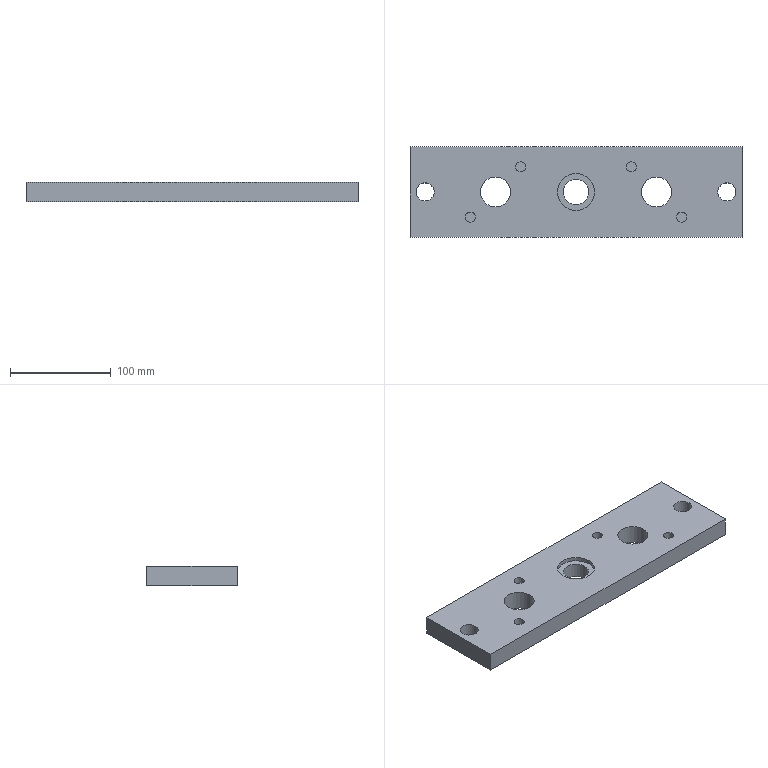Part | NX | features solid 2 | 1 solid | 21 faces | box 330 x 90 x 19 mm | volume 513033 mm3 | plane 11 | cylinder 10 | commonest cylinder face diameters 10 x4 18 x2 30 x2 25 x1 36.704 x1
STEP:
#1=CARTESIAN_POINT('',(-50.,-415.,-181.));
#2=VERTEX_POINT('',#1);
#3=CARTESIAN_POINT('',(-55.,-415.,-181.));
#4=DIRECTION('',(0.,0.,1.));
#5=DIRECTION('',(1.,0.,0.));
#6=AXIS2_PLACEMENT_3D('',#3,#4,#5);
#7=CIRCLE('',#6,5.);
#8=EDGE_CURVE('',#2,#2,#7,.F.);
#9=ORIENTED_EDGE('',*,*,#8,.T.);
#10=EDGE_LOOP('',(#9));
#11=FACE_BOUND('',#10,.T.);
#12=CARTESIAN_POINT('',(60.,-415.,-181.));
#13=VERTEX_POINT('',#12);
#14=CARTESIAN_POINT('',(55.,-415.,-181.));
#15=DIRECTION('',(0.,0.,1.));
#16=DIRECTION('',(1.,0.,0.));
#17=AXIS2_PLACEMENT_3D('',#14,#15,#16);
#18=CIRCLE('',#17,5.);
#19=EDGE_CURVE('',#13,#13,#18,.T.);
#20=ORIENTED_EDGE('',*,*,#19,.F.);
#21=EDGE_LOOP('',(#20));
#22=FACE_BOUND('',#21,.T.);
#23=CARTESIAN_POINT('',(110.,-465.,-181.));
#24=VERTEX_POINT('',#23);
#25=CARTESIAN_POINT('',(105.,-465.,-181.));
#26=DIRECTION('',(0.,0.,1.));
#27=DIRECTION('',(1.,0.,0.));
#28=AXIS2_PLACEMENT_3D('',#25,#26,#27);
#29=CIRCLE('',#28,5.);
#30=EDGE_CURVE('',#24,#24,#29,.T.);
#31=ORIENTED_EDGE('',*,*,#30,.F.);
#32=EDGE_LOOP('',(#31));
#33=FACE_BOUND('',#32,.T.);
#34=CARTESIAN_POINT('',(159.,-440.,-181.));
#35=VERTEX_POINT('',#34);
#36=CARTESIAN_POINT('',(150.,-440.,-181.));
#37=DIRECTION('',(0.,0.,1.));
#38=DIRECTION('',(1.,0.,0.));
#39=AXIS2_PLACEMENT_3D('',#36,#37,#38);
#40=CIRCLE('',#39,9.);
#41=EDGE_CURVE('',#35,#35,#40,.T.);
#42=ORIENTED_EDGE('',*,*,#41,.F.);
#43=EDGE_LOOP('',(#42));
#44=FACE_BOUND('',#43,.T.);
#45=CARTESIAN_POINT('',(-141.,-440.,-181.));
#46=VERTEX_POINT('',#45);
#47=CARTESIAN_POINT('',(-150.,-440.,-181.));
#48=DIRECTION('',(0.,0.,1.));
#49=DIRECTION('',(1.,0.,0.));
#50=AXIS2_PLACEMENT_3D('',#47,#48,#49);
#51=CIRCLE('',#50,9.);
#52=EDGE_CURVE('',#46,#46,#51,.T.);
#53=ORIENTED_EDGE('',*,*,#52,.F.);
#54=EDGE_LOOP('',(#53));
#55=FACE_BOUND('',#54,.T.);
#56=CARTESIAN_POINT('',(-165.,-485.,-181.));
#57=VERTEX_POINT('',#56);
#58=CARTESIAN_POINT('',(-165.,-395.,-181.));
#59=VERTEX_POINT('',#58);
#60=CARTESIAN_POINT('',(-165.,-485.,-181.));
#61=DIRECTION('',(0.,1.,0.));
#62=VECTOR('',#61,1000.);
#63=LINE('',#60,#62);
#64=EDGE_CURVE('',#57,#59,#63,.T.);
#65=ORIENTED_EDGE('',*,*,#64,.F.);
#66=CARTESIAN_POINT('',(165.,-485.,-181.));
#67=VERTEX_POINT('',#66);
#68=CARTESIAN_POINT('',(165.,-485.,-181.));
#69=DIRECTION('',(-1.,0.,0.));
#70=VECTOR('',#69,1000.);
#71=LINE('',#68,#70);
#72=EDGE_CURVE('',#67,#57,#71,.T.);
#73=ORIENTED_EDGE('',*,*,#72,.F.);
#74=CARTESIAN_POINT('',(165.,-395.,-181.));
#75=VERTEX_POINT('',#74);
#76=CARTESIAN_POINT('',(165.,-395.,-181.));
#77=DIRECTION('',(0.,-1.,0.));
#78=VECTOR('',#77,1000.);
#79=LINE('',#76,#78);
#80=EDGE_CURVE('',#75,#67,#79,.T.);
#81=ORIENTED_EDGE('',*,*,#80,.F.);
#82=CARTESIAN_POINT('',(-165.,-395.,-181.));
#83=DIRECTION('',(1.,0.,0.));
#84=VECTOR('',#83,1000.);
#85=LINE('',#82,#84);
#86=EDGE_CURVE('',#59,#75,#85,.T.);
#87=ORIENTED_EDGE('',*,*,#86,.F.);
#88=EDGE_LOOP('',(#65,#73,#81,#87));
#89=FACE_BOUND('',#88,.T.);
#90=CARTESIAN_POINT('',(-65.,-440.,-181.));
#91=VERTEX_POINT('',#90);
#92=CARTESIAN_POINT('',(-80.,-440.,-181.));
#93=DIRECTION('',(0.,0.,1.));
#94=DIRECTION('',(1.,0.,0.));
#95=AXIS2_PLACEMENT_3D('',#92,#93,#94);
#96=CIRCLE('',#95,15.);
#97=EDGE_CURVE('',#91,#91,#96,.T.);
#98=ORIENTED_EDGE('',*,*,#97,.F.);
#99=EDGE_LOOP('',(#98));
#100=FACE_BOUND('',#99,.T.);
#101=CARTESIAN_POINT('',(95.,-440.,-181.));
#102=VERTEX_POINT('',#101);
#103=CARTESIAN_POINT('',(80.,-440.,-181.));
#104=DIRECTION('',(0.,0.,1.));
#105=DIRECTION('',(1.,0.,0.));
#106=AXIS2_PLACEMENT_3D('',#103,#104,#105);
#107=CIRCLE('',#106,15.);
#108=EDGE_CURVE('',#102,#102,#107,.T.);
#109=ORIENTED_EDGE('',*,*,#108,.F.);
#110=EDGE_LOOP('',(#109));
#111=FACE_BOUND('',#110,.T.);
#112=CARTESIAN_POINT('',(18.352,-440.,-181.));
#113=VERTEX_POINT('',#112);
#114=CARTESIAN_POINT('',(0.,-440.,-181.));
#115=DIRECTION('',(0.,0.,1.));
#116=DIRECTION('',(1.,0.,0.));
#117=AXIS2_PLACEMENT_3D('',#114,#115,#116);
#118=CIRCLE('',#117,18.352);
#119=EDGE_CURVE('',#113,#113,#118,.T.);
#120=ORIENTED_EDGE('',*,*,#119,.F.);
#121=EDGE_LOOP('',(#120));
#122=FACE_BOUND('',#121,.T.);
#123=CARTESIAN_POINT('',(-100.,-465.,-181.));
#124=VERTEX_POINT('',#123);
#125=CARTESIAN_POINT('',(-105.,-465.,-181.));
#126=DIRECTION('',(0.,0.,1.));
#127=DIRECTION('',(1.,0.,0.));
#128=AXIS2_PLACEMENT_3D('',#125,#126,#127);
#129=CIRCLE('',#128,5.);
#130=EDGE_CURVE('',#124,#124,#129,.F.);
#131=ORIENTED_EDGE('',*,*,#130,.T.);
#132=EDGE_LOOP('',(#131));
#133=FACE_BOUND('',#132,.T.);
#134=CARTESIAN_POINT('',(-165.,-485.,-181.));
#135=DIRECTION('',(0.,0.,-1.));
#136=DIRECTION('',(1.,0.,0.));
#137=AXIS2_PLACEMENT_3D('',#134,#135,#136);
#138=PLANE('',#137);
#139=ADVANCED_FACE('',(#11,#22,#33,#44,#55,#89,#100,#111,#122,#133),#138,.F.);
#140=ORIENTED_EDGE('',*,*,#64,.T.);
#141=CARTESIAN_POINT('',(-165.,-395.,-200.));
#142=VERTEX_POINT('',#141);
#143=CARTESIAN_POINT('',(-165.,-395.,-200.));
#144=DIRECTION('',(0.,0.,1.));
#145=VECTOR('',#144,1000.);
#146=LINE('',#143,#145);
#147=EDGE_CURVE('',#142,#59,#146,.T.);
#148=ORIENTED_EDGE('',*,*,#147,.F.);
#149=CARTESIAN_POINT('',(-165.,-485.,-200.));
#150=VERTEX_POINT('',#149);
#151=CARTESIAN_POINT('',(-165.,-485.,-200.));
#152=DIRECTION('',(0.,1.,0.));
#153=VECTOR('',#152,1000.);
#154=LINE('',#151,#153);
#155=EDGE_CURVE('',#150,#142,#154,.T.);
#156=ORIENTED_EDGE('',*,*,#155,.F.);
#157=CARTESIAN_POINT('',(-165.,-485.,-200.));
#158=DIRECTION('',(0.,0.,1.));
#159=VECTOR('',#158,1000.);
#160=LINE('',#157,#159);
#161=EDGE_CURVE('',#150,#57,#160,.T.);
#162=ORIENTED_EDGE('',*,*,#161,.T.);
#163=EDGE_LOOP('',(#140,#148,#156,#162));
#164=FACE_BOUND('',#163,.T.);
#165=CARTESIAN_POINT('',(-165.,-485.,-200.));
#166=DIRECTION('',(-1.,0.,0.));
#167=DIRECTION('',(0.,0.,-1.));
#168=AXIS2_PLACEMENT_3D('',#165,#166,#167);
#169=PLANE('',#168);
#170=ADVANCED_FACE('',(#164),#169,.T.);
#171=ORIENTED_EDGE('',*,*,#86,.T.);
#172=CARTESIAN_POINT('',(165.,-395.,-200.));
#173=VERTEX_POINT('',#172);
#174=CARTESIAN_POINT('',(165.,-395.,-200.));
#175=DIRECTION('',(0.,0.,1.));
#176=VECTOR('',#175,1000.);
#177=LINE('',#174,#176);
#178=EDGE_CURVE('',#173,#75,#177,.T.);
#179=ORIENTED_EDGE('',*,*,#178,.F.);
#180=CARTESIAN_POINT('',(-165.,-395.,-200.));
#181=DIRECTION('',(1.,0.,0.));
#182=VECTOR('',#181,1000.);
#183=LINE('',#180,#182);
#184=EDGE_CURVE('',#142,#173,#183,.T.);
#185=ORIENTED_EDGE('',*,*,#184,.F.);
#186=ORIENTED_EDGE('',*,*,#147,.T.);
#187=EDGE_LOOP('',(#171,#179,#185,#186));
#188=FACE_BOUND('',#187,.T.);
#189=CARTESIAN_POINT('',(-165.,-395.,-200.));
#190=DIRECTION('',(0.,1.,0.));
#191=DIRECTION('',(-1.,0.,0.));
#192=AXIS2_PLACEMENT_3D('',#189,#190,#191);
#193=PLANE('',#192);
#194=ADVANCED_FACE('',(#188),#193,.T.);
#195=ORIENTED_EDGE('',*,*,#80,.T.);
#196=CARTESIAN_POINT('',(165.,-485.,-200.));
#197=VERTEX_POINT('',#196);
#198=CARTESIAN_POINT('',(165.,-485.,-200.));
#199=DIRECTION('',(0.,0.,1.));
#200=VECTOR('',#199,1000.);
#201=LINE('',#198,#200);
#202=EDGE_CURVE('',#197,#67,#201,.T.);
#203=ORIENTED_EDGE('',*,*,#202,.F.);
#204=CARTESIAN_POINT('',(165.,-395.,-200.));
#205=DIRECTION('',(0.,-1.,0.));
#206=VECTOR('',#205,1000.);
#207=LINE('',#204,#206);
#208=EDGE_CURVE('',#173,#197,#207,.T.);
#209=ORIENTED_EDGE('',*,*,#208,.F.);
#210=ORIENTED_EDGE('',*,*,#178,.T.);
#211=EDGE_LOOP('',(#195,#203,#209,#210));
#212=FACE_BOUND('',#211,.T.);
#213=CARTESIAN_POINT('',(165.,-395.,-200.));
#214=DIRECTION('',(1.,0.,0.));
#215=DIRECTION('',(0.,0.,1.));
#216=AXIS2_PLACEMENT_3D('',#213,#214,#215);
#217=PLANE('',#216);
#218=ADVANCED_FACE('',(#212),#217,.T.);
#219=CARTESIAN_POINT('',(12.5,-440.,-185.));
#220=VERTEX_POINT('',#219);
#221=CARTESIAN_POINT('',(0.,-440.,-185.));
#222=DIRECTION('',(0.,0.,1.));
#223=DIRECTION('',(1.,0.,0.));
#224=AXIS2_PLACEMENT_3D('',#221,#222,#223);
#225=CIRCLE('',#224,12.5);
#226=EDGE_CURVE('',#220,#220,#225,.T.);
#227=ORIENTED_EDGE('',*,*,#226,.T.);
#228=EDGE_LOOP('',(#227));
#229=FACE_BOUND('',#228,.T.);
#230=CARTESIAN_POINT('',(12.5,-440.,-200.));
#231=VERTEX_POINT('',#230);
#232=CARTESIAN_POINT('',(0.,-440.,-200.));
#233=DIRECTION('',(0.,0.,1.));
#234=DIRECTION('',(1.,0.,0.));
#235=AXIS2_PLACEMENT_3D('',#232,#233,#234);
#236=CIRCLE('',#235,12.5);
#237=EDGE_CURVE('',#231,#231,#236,.T.);
#238=ORIENTED_EDGE('',*,*,#237,.F.);
#239=EDGE_LOOP('',(#238));
#240=FACE_BOUND('',#239,.T.);
#241=CARTESIAN_POINT('',(0.,-440.,-200.));
#242=DIRECTION('',(0.,0.,1.));
#243=DIRECTION('',(-1.,0.,0.));
#244=AXIS2_PLACEMENT_3D('',#241,#242,#243);
#245=CYLINDRICAL_SURFACE('',#244,12.5);
#246=ADVANCED_FACE('',(#229,#240),#245,.F.);
#247=CARTESIAN_POINT('',(-141.,-440.,-200.));
#248=VERTEX_POINT('',#247);
#249=CARTESIAN_POINT('',(-150.,-440.,-200.));
#250=DIRECTION('',(0.,0.,1.));
#251=DIRECTION('',(1.,0.,0.));
#252=AXIS2_PLACEMENT_3D('',#249,#250,#251);
#253=CIRCLE('',#252,9.);
#254=EDGE_CURVE('',#248,#248,#253,.T.);
#255=ORIENTED_EDGE('',*,*,#254,.F.);
#256=EDGE_LOOP('',(#255));
#257=FACE_BOUND('',#256,.T.);
#258=ORIENTED_EDGE('',*,*,#52,.T.);
#259=EDGE_LOOP('',(#258));
#260=FACE_BOUND('',#259,.T.);
#261=CARTESIAN_POINT('',(-150.,-440.,-200.));
#262=DIRECTION('',(0.,0.,1.));
#263=DIRECTION('',(-1.,0.,0.));
#264=AXIS2_PLACEMENT_3D('',#261,#262,#263);
#265=CYLINDRICAL_SURFACE('',#264,9.);
#266=ADVANCED_FACE('',(#257,#260),#265,.F.);
#267=ORIENTED_EDGE('',*,*,#72,.T.);
#268=ORIENTED_EDGE('',*,*,#161,.F.);
#269=CARTESIAN_POINT('',(165.,-485.,-200.));
#270=DIRECTION('',(-1.,0.,0.));
#271=VECTOR('',#270,1000.);
#272=LINE('',#269,#271);
#273=EDGE_CURVE('',#197,#150,#272,.T.);
#274=ORIENTED_EDGE('',*,*,#273,.F.);
#275=ORIENTED_EDGE('',*,*,#202,.T.);
#276=EDGE_LOOP('',(#267,#268,#274,#275));
#277=FACE_BOUND('',#276,.T.);
#278=CARTESIAN_POINT('',(165.,-485.,-200.));
#279=DIRECTION('',(0.,-1.,0.));
#280=DIRECTION('',(1.,0.,0.));
#281=AXIS2_PLACEMENT_3D('',#278,#279,#280);
#282=PLANE('',#281);
#283=ADVANCED_FACE('',(#277),#282,.T.);
#284=CARTESIAN_POINT('',(-65.,-440.,-200.));
#285=VERTEX_POINT('',#284);
#286=CARTESIAN_POINT('',(-80.,-440.,-200.));
#287=DIRECTION('',(0.,0.,1.));
#288=DIRECTION('',(1.,0.,0.));
#289=AXIS2_PLACEMENT_3D('',#286,#287,#288);
#290=CIRCLE('',#289,15.);
#291=EDGE_CURVE('',#285,#285,#290,.T.);
#292=ORIENTED_EDGE('',*,*,#291,.F.);
#293=EDGE_LOOP('',(#292));
#294=FACE_BOUND('',#293,.T.);
#295=ORIENTED_EDGE('',*,*,#97,.T.);
#296=EDGE_LOOP('',(#295));
#297=FACE_BOUND('',#296,.T.);
#298=CARTESIAN_POINT('',(-80.,-440.,-200.));
#299=DIRECTION('',(0.,0.,1.));
#300=DIRECTION('',(-1.,0.,0.));
#301=AXIS2_PLACEMENT_3D('',#298,#299,#300);
#302=CYLINDRICAL_SURFACE('',#301,15.);
#303=ADVANCED_FACE('',(#294,#297),#302,.F.);
#304=CARTESIAN_POINT('',(95.,-440.,-200.));
#305=VERTEX_POINT('',#304);
#306=CARTESIAN_POINT('',(80.,-440.,-200.));
#307=DIRECTION('',(0.,0.,1.));
#308=DIRECTION('',(1.,0.,0.));
#309=AXIS2_PLACEMENT_3D('',#306,#307,#308);
#310=CIRCLE('',#309,15.);
#311=EDGE_CURVE('',#305,#305,#310,.T.);
#312=ORIENTED_EDGE('',*,*,#311,.F.);
#313=EDGE_LOOP('',(#312));
#314=FACE_BOUND('',#313,.T.);
#315=ORIENTED_EDGE('',*,*,#108,.T.);
#316=EDGE_LOOP('',(#315));
#317=FACE_BOUND('',#316,.T.);
#318=CARTESIAN_POINT('',(80.,-440.,-200.));
#319=DIRECTION('',(0.,0.,1.));
#320=DIRECTION('',(-1.,0.,0.));
#321=AXIS2_PLACEMENT_3D('',#318,#319,#320);
#322=CYLINDRICAL_SURFACE('',#321,15.);
#323=ADVANCED_FACE('',(#314,#317),#322,.F.);
#324=CARTESIAN_POINT('',(159.,-440.,-200.));
#325=VERTEX_POINT('',#324);
#326=CARTESIAN_POINT('',(150.,-440.,-200.));
#327=DIRECTION('',(0.,0.,1.));
#328=DIRECTION('',(1.,0.,0.));
#329=AXIS2_PLACEMENT_3D('',#326,#327,#328);
#330=CIRCLE('',#329,9.);
#331=EDGE_CURVE('',#325,#325,#330,.T.);
#332=ORIENTED_EDGE('',*,*,#331,.F.);
#333=EDGE_LOOP('',(#332));
#334=FACE_BOUND('',#333,.T.);
#335=ORIENTED_EDGE('',*,*,#41,.T.);
#336=EDGE_LOOP('',(#335));
#337=FACE_BOUND('',#336,.T.);
#338=CARTESIAN_POINT('',(150.,-440.,-200.));
#339=DIRECTION('',(0.,0.,1.));
#340=DIRECTION('',(-1.,0.,0.));
#341=AXIS2_PLACEMENT_3D('',#338,#339,#340);
#342=CYLINDRICAL_SURFACE('',#341,9.);
#343=ADVANCED_FACE('',(#334,#337),#342,.F.);
#344=ORIENTED_EDGE('',*,*,#311,.T.);
#345=EDGE_LOOP('',(#344));
#346=FACE_BOUND('',#345,.T.);
#347=ORIENTED_EDGE('',*,*,#291,.T.);
#348=EDGE_LOOP('',(#347));
#349=FACE_BOUND('',#348,.T.);
#350=ORIENTED_EDGE('',*,*,#155,.T.);
#351=ORIENTED_EDGE('',*,*,#184,.T.);
#352=ORIENTED_EDGE('',*,*,#208,.T.);
#353=ORIENTED_EDGE('',*,*,#273,.T.);
#354=EDGE_LOOP('',(#350,#351,#352,#353));
#355=FACE_BOUND('',#354,.T.);
#356=ORIENTED_EDGE('',*,*,#254,.T.);
#357=EDGE_LOOP('',(#356));
#358=FACE_BOUND('',#357,.T.);
#359=ORIENTED_EDGE('',*,*,#237,.T.);
#360=EDGE_LOOP('',(#359));
#361=FACE_BOUND('',#360,.T.);
#362=ORIENTED_EDGE('',*,*,#331,.T.);
#363=EDGE_LOOP('',(#362));
#364=FACE_BOUND('',#363,.T.);
#365=CARTESIAN_POINT('',(-165.,-485.,-200.));
#366=DIRECTION('',(0.,0.,-1.));
#367=DIRECTION('',(1.,0.,0.));
#368=AXIS2_PLACEMENT_3D('',#365,#366,#367);
#369=PLANE('',#368);
#370=ADVANCED_FACE('',(#346,#349,#355,#358,#361,#364),#369,.T.);
#371=CARTESIAN_POINT('',(18.352,-440.,-185.));
#372=VERTEX_POINT('',#371);
#373=CARTESIAN_POINT('',(0.,-440.,-185.));
#374=DIRECTION('',(0.,0.,1.));
#375=DIRECTION('',(1.,0.,0.));
#376=AXIS2_PLACEMENT_3D('',#373,#374,#375);
#377=CIRCLE('',#376,18.352);
#378=EDGE_CURVE('',#372,#372,#377,.T.);
#379=ORIENTED_EDGE('',*,*,#378,.F.);
#380=EDGE_LOOP('',(#379));
#381=FACE_BOUND('',#380,.T.);
#382=ORIENTED_EDGE('',*,*,#119,.T.);
#383=EDGE_LOOP('',(#382));
#384=FACE_BOUND('',#383,.T.);
#385=CARTESIAN_POINT('',(0.,-440.,-185.));
#386=DIRECTION('',(0.,0.,1.));
#387=DIRECTION('',(-1.,0.,0.));
#388=AXIS2_PLACEMENT_3D('',#385,#386,#387);
#389=CYLINDRICAL_SURFACE('',#388,18.352);
#390=ADVANCED_FACE('',(#381,#384),#389,.F.);
#391=ORIENTED_EDGE('',*,*,#226,.F.);
#392=EDGE_LOOP('',(#391));
#393=FACE_BOUND('',#392,.T.);
#394=ORIENTED_EDGE('',*,*,#378,.T.);
#395=EDGE_LOOP('',(#394));
#396=FACE_BOUND('',#395,.T.);
#397=CARTESIAN_POINT('',(0.,-440.,-185.));
#398=DIRECTION('',(0.,0.,-1.));
#399=DIRECTION('',(1.,0.,0.));
#400=AXIS2_PLACEMENT_3D('',#397,#398,#399);
#401=PLANE('',#400);
#402=ADVANCED_FACE('',(#393,#396),#401,.F.);
#403=CARTESIAN_POINT('',(100.,-465.,-191.));
#404=VERTEX_POINT('',#403);
#405=CARTESIAN_POINT('',(105.,-465.,-191.));
#406=DIRECTION('',(0.,0.,-1.));
#407=DIRECTION('',(-1.,0.,0.));
#408=AXIS2_PLACEMENT_3D('',#405,#406,#407);
#409=CIRCLE('',#408,5.);
#410=EDGE_CURVE('',#404,#404,#409,.T.);
#411=ORIENTED_EDGE('',*,*,#410,.T.);
#412=EDGE_LOOP('',(#411));
#413=FACE_BOUND('',#412,.T.);
#414=ORIENTED_EDGE('',*,*,#30,.T.);
#415=EDGE_LOOP('',(#414));
#416=FACE_BOUND('',#415,.T.);
#417=CARTESIAN_POINT('',(105.,-465.,-191.));
#418=DIRECTION('',(0.,0.,1.));
#419=DIRECTION('',(-1.,0.,0.));
#420=AXIS2_PLACEMENT_3D('',#417,#418,#419);
#421=CYLINDRICAL_SURFACE('',#420,5.);
#422=ADVANCED_FACE('',(#413,#416),#421,.F.);
#423=ORIENTED_EDGE('',*,*,#410,.F.);
#424=EDGE_LOOP('',(#423));
#425=FACE_BOUND('',#424,.T.);
#426=CARTESIAN_POINT('',(105.,-465.,-191.));
#427=DIRECTION('',(0.,0.,1.));
#428=DIRECTION('',(-1.,0.,0.));
#429=AXIS2_PLACEMENT_3D('',#426,#427,#428);
#430=PLANE('',#429);
#431=ADVANCED_FACE('',(#425),#430,.T.);
#432=CARTESIAN_POINT('',(50.,-415.,-191.));
#433=VERTEX_POINT('',#432);
#434=CARTESIAN_POINT('',(55.,-415.,-191.));
#435=DIRECTION('',(0.,0.,-1.));
#436=DIRECTION('',(-1.,0.,0.));
#437=AXIS2_PLACEMENT_3D('',#434,#435,#436);
#438=CIRCLE('',#437,5.);
#439=EDGE_CURVE('',#433,#433,#438,.T.);
#440=ORIENTED_EDGE('',*,*,#439,.T.);
#441=EDGE_LOOP('',(#440));
#442=FACE_BOUND('',#441,.T.);
#443=ORIENTED_EDGE('',*,*,#19,.T.);
#444=EDGE_LOOP('',(#443));
#445=FACE_BOUND('',#444,.T.);
#446=CARTESIAN_POINT('',(55.,-415.,-191.));
#447=DIRECTION('',(0.,0.,1.));
#448=DIRECTION('',(-1.,0.,0.));
#449=AXIS2_PLACEMENT_3D('',#446,#447,#448);
#450=CYLINDRICAL_SURFACE('',#449,5.);
#451=ADVANCED_FACE('',(#442,#445),#450,.F.);
#452=ORIENTED_EDGE('',*,*,#439,.F.);
#453=EDGE_LOOP('',(#452));
#454=FACE_BOUND('',#453,.T.);
#455=CARTESIAN_POINT('',(55.,-415.,-191.));
#456=DIRECTION('',(0.,0.,1.));
#457=DIRECTION('',(-1.,0.,0.));
#458=AXIS2_PLACEMENT_3D('',#455,#456,#457);
#459=PLANE('',#458);
#460=ADVANCED_FACE('',(#454),#459,.T.);
#461=CARTESIAN_POINT('',(-50.,-415.,-191.));
#462=VERTEX_POINT('',#461);
#463=CARTESIAN_POINT('',(-55.,-415.,-191.));
#464=DIRECTION('',(0.,0.,1.));
#465=DIRECTION('',(1.,0.,0.));
#466=AXIS2_PLACEMENT_3D('',#463,#464,#465);
#467=CIRCLE('',#466,5.);
#468=EDGE_CURVE('',#462,#462,#467,.T.);
#469=ORIENTED_EDGE('',*,*,#468,.F.);
#470=EDGE_LOOP('',(#469));
#471=FACE_BOUND('',#470,.T.);
#472=ORIENTED_EDGE('',*,*,#8,.F.);
#473=EDGE_LOOP('',(#472));
#474=FACE_BOUND('',#473,.T.);
#475=CARTESIAN_POINT('',(-55.,-415.,-191.));
#476=DIRECTION('',(0.,0.,1.));
#477=DIRECTION('',(-1.,0.,0.));
#478=AXIS2_PLACEMENT_3D('',#475,#476,#477);
#479=CYLINDRICAL_SURFACE('',#478,5.);
#480=ADVANCED_FACE('',(#471,#474),#479,.F.);
#481=ORIENTED_EDGE('',*,*,#468,.T.);
#482=EDGE_LOOP('',(#481));
#483=FACE_BOUND('',#482,.T.);
#484=CARTESIAN_POINT('',(-55.,-415.,-191.));
#485=DIRECTION('',(0.,0.,-1.));
#486=DIRECTION('',(1.,0.,0.));
#487=AXIS2_PLACEMENT_3D('',#484,#485,#486);
#488=PLANE('',#487);
#489=ADVANCED_FACE('',(#483),#488,.F.);
#490=CARTESIAN_POINT('',(-100.,-465.,-191.));
#491=VERTEX_POINT('',#490);
#492=CARTESIAN_POINT('',(-105.,-465.,-191.));
#493=DIRECTION('',(0.,0.,1.));
#494=DIRECTION('',(1.,0.,0.));
#495=AXIS2_PLACEMENT_3D('',#492,#493,#494);
#496=CIRCLE('',#495,5.);
#497=EDGE_CURVE('',#491,#491,#496,.T.);
#498=ORIENTED_EDGE('',*,*,#497,.F.);
#499=EDGE_LOOP('',(#498));
#500=FACE_BOUND('',#499,.T.);
#501=ORIENTED_EDGE('',*,*,#130,.F.);
#502=EDGE_LOOP('',(#501));
#503=FACE_BOUND('',#502,.T.);
#504=CARTESIAN_POINT('',(-105.,-465.,-191.));
#505=DIRECTION('',(0.,0.,1.));
#506=DIRECTION('',(-1.,0.,0.));
#507=AXIS2_PLACEMENT_3D('',#504,#505,#506);
#508=CYLINDRICAL_SURFACE('',#507,5.);
#509=ADVANCED_FACE('',(#500,#503),#508,.F.);
#510=ORIENTED_EDGE('',*,*,#497,.T.);
#511=EDGE_LOOP('',(#510));
#512=FACE_BOUND('',#511,.T.);
#513=CARTESIAN_POINT('',(-105.,-465.,-191.));
#514=DIRECTION('',(0.,0.,-1.));
#515=DIRECTION('',(1.,0.,0.));
#516=AXIS2_PLACEMENT_3D('',#513,#514,#515);
#517=PLANE('',#516);
#518=ADVANCED_FACE('',(#512),#517,.F.);
#519=CLOSED_SHELL('',(#139,#170,#194,#218,#246,#266,#283,#303,#323,#343,#370,#390,#402,#422,#431,#451,#460,#480,#489,#509,#518));
#520=MANIFOLD_SOLID_BREP('',#519);
#521=(LENGTH_UNIT()NAMED_UNIT(*)SI_UNIT(.MILLI.,.METRE.));
#522=UNCERTAINTY_MEASURE_WITH_UNIT(LENGTH_MEASURE(0.00001),#521,'','');
#523=(NAMED_UNIT(*)PLANE_ANGLE_UNIT()SI_UNIT($,.RADIAN.));
#524=(NAMED_UNIT(*)SI_UNIT($,.STERADIAN.)SOLID_ANGLE_UNIT());
#525=(GEOMETRIC_REPRESENTATION_CONTEXT(3)GLOBAL_UNCERTAINTY_ASSIGNED_CONTEXT((#522))GLOBAL_UNIT_ASSIGNED_CONTEXT((#521,#523,#524))REPRESENTATION_CONTEXT('',''));
#526=ADVANCED_BREP_SHAPE_REPRESENTATION('',(#520),#525);